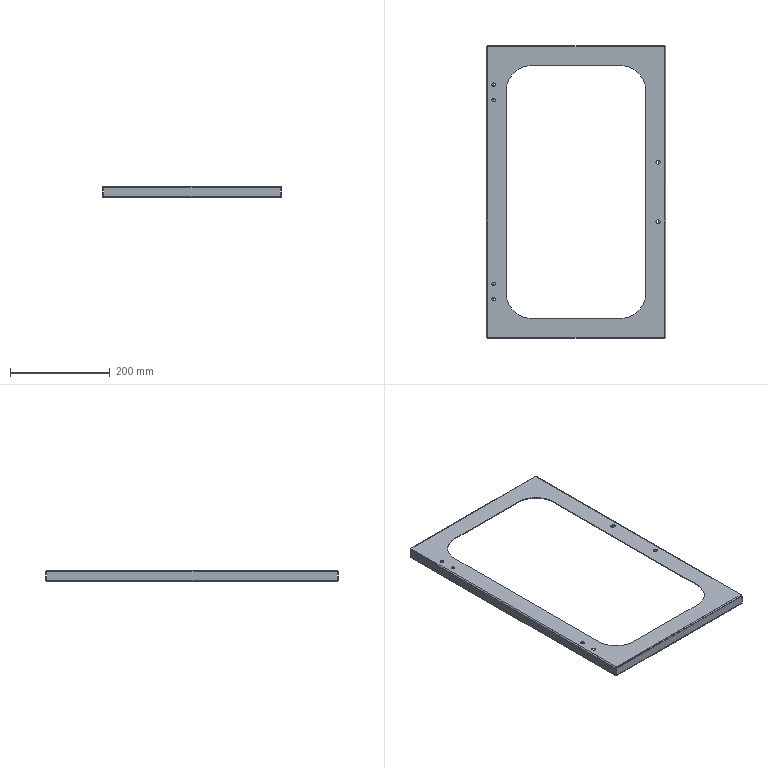Part | STEP file | Sheet metal front door | 1 solid | 90 faces | box 360 x 588 x 21.5 mm | volume 195995 mm3 | plane 42 | cylinder 32 | spline 16 | commonest cylinder face diameters 2 x8 5 x8 7 x8 8.5 x4 100 x4